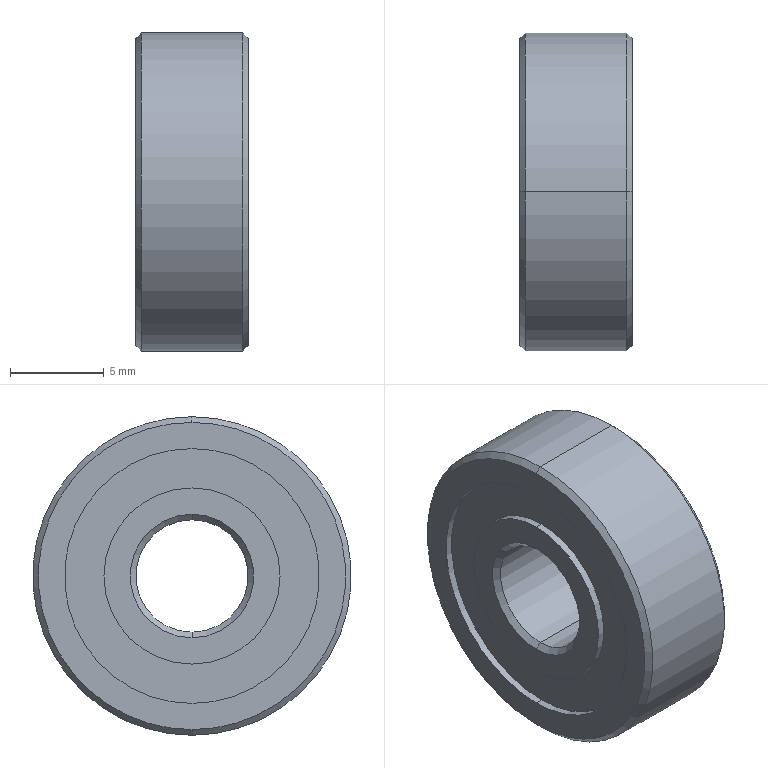Part | SolidWorks | features BaseBody 1 | 1 solid | 26 faces | box 6 x 17 x 17 mm | volume 1125 mm3 | cylinder 12 | cone 8 | plane 6 | commonest cylinder face diameters 9.4 x4 13.6 x4 6 x2 17 x2
STEP:
#1=CARTESIAN_POINT('',(2.7,0.,8.5));
#2=VERTEX_POINT('',#1);
#3=CARTESIAN_POINT('',(2.7,0.,-8.5));
#4=VERTEX_POINT('',#3);
#5=CARTESIAN_POINT('',(2.7,0.,0.));
#6=DIRECTION('',(-1.,0.,0.));
#7=DIRECTION('',(0.,0.,1.));
#8=AXIS2_PLACEMENT_3D('',#5,#6,#7);
#9=CIRCLE('',#8,8.5);
#10=EDGE_CURVE('',#2,#4,#9,.T.);
#11=ORIENTED_EDGE('',*,*,#10,.T.);
#12=CARTESIAN_POINT('',(-2.7,0.,-8.5));
#13=VERTEX_POINT('',#12);
#14=CARTESIAN_POINT('',(3.,0.,-8.5));
#15=DIRECTION('',(-1.,0.,0.));
#16=VECTOR('',#15,1000.);
#17=LINE('',#14,#16);
#18=EDGE_CURVE('',#4,#13,#17,.T.);
#19=ORIENTED_EDGE('',*,*,#18,.T.);
#20=CARTESIAN_POINT('',(-2.7,0.,8.5));
#21=VERTEX_POINT('',#20);
#22=CARTESIAN_POINT('',(-2.7,0.,0.));
#23=DIRECTION('',(1.,0.,0.));
#24=DIRECTION('',(0.,0.,1.));
#25=AXIS2_PLACEMENT_3D('',#22,#23,#24);
#26=CIRCLE('',#25,8.5);
#27=EDGE_CURVE('',#13,#21,#26,.T.);
#28=ORIENTED_EDGE('',*,*,#27,.T.);
#29=CARTESIAN_POINT('',(3.,0.,8.5));
#30=DIRECTION('',(-1.,0.,0.));
#31=VECTOR('',#30,1000.);
#32=LINE('',#29,#31);
#33=EDGE_CURVE('',#2,#21,#32,.T.);
#34=ORIENTED_EDGE('',*,*,#33,.F.);
#35=EDGE_LOOP('',(#11,#19,#28,#34));
#36=FACE_OUTER_BOUND('',#35,.T.);
#37=CARTESIAN_POINT('',(3.,0.,0.));
#38=DIRECTION('',(-1.,0.,0.));
#39=DIRECTION('',(0.,0.,1.));
#40=AXIS2_PLACEMENT_3D('',#37,#38,#39);
#41=CYLINDRICAL_SURFACE('',#40,8.5);
#42=ADVANCED_FACE('',(#36),#41,.T.);
#43=CARTESIAN_POINT('',(3.,0.,8.2));
#44=VERTEX_POINT('',#43);
#45=CARTESIAN_POINT('',(3.,0.,-8.2));
#46=VERTEX_POINT('',#45);
#47=CARTESIAN_POINT('',(3.,0.,0.));
#48=DIRECTION('',(-1.,0.,0.));
#49=DIRECTION('',(0.,0.,1.));
#50=AXIS2_PLACEMENT_3D('',#47,#48,#49);
#51=CIRCLE('',#50,8.2);
#52=EDGE_CURVE('',#44,#46,#51,.T.);
#53=ORIENTED_EDGE('',*,*,#52,.T.);
#54=CARTESIAN_POINT('',(2.7,0.,-8.5));
#55=DIRECTION('',(-0.7071,0.,-0.7071));
#56=VECTOR('',#55,1000.);
#57=LINE('',#54,#56);
#58=EDGE_CURVE('',#46,#4,#57,.T.);
#59=ORIENTED_EDGE('',*,*,#58,.T.);
#60=ORIENTED_EDGE('',*,*,#10,.F.);
#61=CARTESIAN_POINT('',(2.7,0.,8.5));
#62=DIRECTION('',(-0.7071,0.,0.7071));
#63=VECTOR('',#62,1000.);
#64=LINE('',#61,#63);
#65=EDGE_CURVE('',#44,#2,#64,.T.);
#66=ORIENTED_EDGE('',*,*,#65,.F.);
#67=EDGE_LOOP('',(#53,#59,#60,#66));
#68=FACE_OUTER_BOUND('',#67,.T.);
#69=CARTESIAN_POINT('',(2.7,0.,0.));
#70=DIRECTION('',(-1.,0.,0.));
#71=DIRECTION('',(0.,0.,1.));
#72=AXIS2_PLACEMENT_3D('',#69,#70,#71);
#73=CONICAL_SURFACE('',#72,8.5,0.7854);
#74=ADVANCED_FACE('',(#68),#73,.T.);
#75=CARTESIAN_POINT('',(-3.,0.,-8.2));
#76=VERTEX_POINT('',#75);
#77=CARTESIAN_POINT('',(-3.,0.,8.2));
#78=VERTEX_POINT('',#77);
#79=CARTESIAN_POINT('',(-3.,0.,0.));
#80=DIRECTION('',(1.,0.,0.));
#81=DIRECTION('',(0.,0.,-1.));
#82=AXIS2_PLACEMENT_3D('',#79,#80,#81);
#83=CIRCLE('',#82,8.2);
#84=EDGE_CURVE('',#76,#78,#83,.T.);
#85=ORIENTED_EDGE('',*,*,#84,.T.);
#86=CARTESIAN_POINT('',(-2.7,0.,8.5));
#87=DIRECTION('',(0.7071,0.,0.7071));
#88=VECTOR('',#87,1000.);
#89=LINE('',#86,#88);
#90=EDGE_CURVE('',#78,#21,#89,.T.);
#91=ORIENTED_EDGE('',*,*,#90,.T.);
#92=ORIENTED_EDGE('',*,*,#27,.F.);
#93=CARTESIAN_POINT('',(-2.7,0.,-8.5));
#94=DIRECTION('',(0.7071,0.,-0.7071));
#95=VECTOR('',#94,1000.);
#96=LINE('',#93,#95);
#97=EDGE_CURVE('',#76,#13,#96,.T.);
#98=ORIENTED_EDGE('',*,*,#97,.F.);
#99=EDGE_LOOP('',(#85,#91,#92,#98));
#100=FACE_OUTER_BOUND('',#99,.T.);
#101=CARTESIAN_POINT('',(-2.7,0.,0.));
#102=DIRECTION('',(1.,0.,0.));
#103=DIRECTION('',(0.,0.,-1.));
#104=AXIS2_PLACEMENT_3D('',#101,#102,#103);
#105=CONICAL_SURFACE('',#104,8.5,0.7854);
#106=ADVANCED_FACE('',(#100),#105,.T.);
#107=CARTESIAN_POINT('',(3.,0.,-6.8));
#108=VERTEX_POINT('',#107);
#109=CARTESIAN_POINT('',(3.,0.,6.8));
#110=VERTEX_POINT('',#109);
#111=CARTESIAN_POINT('',(3.,0.,0.));
#112=DIRECTION('',(-1.,0.,0.));
#113=DIRECTION('',(0.,0.,1.));
#114=AXIS2_PLACEMENT_3D('',#111,#112,#113);
#115=CIRCLE('',#114,6.8);
#116=EDGE_CURVE('',#108,#110,#115,.T.);
#117=ORIENTED_EDGE('',*,*,#116,.F.);
#118=CARTESIAN_POINT('',(2.6,0.,-6.8));
#119=VERTEX_POINT('',#118);
#120=CARTESIAN_POINT('',(3.,0.,-6.8));
#121=DIRECTION('',(-1.,0.,0.));
#122=VECTOR('',#121,1000.);
#123=LINE('',#120,#122);
#124=EDGE_CURVE('',#108,#119,#123,.T.);
#125=ORIENTED_EDGE('',*,*,#124,.T.);
#126=CARTESIAN_POINT('',(2.6,0.,6.8));
#127=VERTEX_POINT('',#126);
#128=CARTESIAN_POINT('',(2.6,0.,0.));
#129=DIRECTION('',(1.,0.,0.));
#130=DIRECTION('',(0.,0.,1.));
#131=AXIS2_PLACEMENT_3D('',#128,#129,#130);
#132=CIRCLE('',#131,6.8);
#133=EDGE_CURVE('',#127,#119,#132,.T.);
#134=ORIENTED_EDGE('',*,*,#133,.F.);
#135=CARTESIAN_POINT('',(3.,0.,6.8));
#136=DIRECTION('',(-1.,0.,0.));
#137=VECTOR('',#136,1000.);
#138=LINE('',#135,#137);
#139=EDGE_CURVE('',#110,#127,#138,.T.);
#140=ORIENTED_EDGE('',*,*,#139,.F.);
#141=EDGE_LOOP('',(#117,#125,#134,#140));
#142=FACE_OUTER_BOUND('',#141,.T.);
#143=CARTESIAN_POINT('',(3.,0.,0.));
#144=DIRECTION('',(-1.,0.,0.));
#145=DIRECTION('',(0.,0.,1.));
#146=AXIS2_PLACEMENT_3D('',#143,#144,#145);
#147=CYLINDRICAL_SURFACE('',#146,6.8);
#148=ADVANCED_FACE('',(#142),#147,.F.);
#149=CARTESIAN_POINT('',(-2.6,0.,-6.8));
#150=VERTEX_POINT('',#149);
#151=CARTESIAN_POINT('',(-2.6,0.,6.8));
#152=VERTEX_POINT('',#151);
#153=CARTESIAN_POINT('',(-2.6,0.,0.));
#154=DIRECTION('',(-1.,0.,0.));
#155=DIRECTION('',(0.,0.,1.));
#156=AXIS2_PLACEMENT_3D('',#153,#154,#155);
#157=CIRCLE('',#156,6.8);
#158=EDGE_CURVE('',#150,#152,#157,.T.);
#159=ORIENTED_EDGE('',*,*,#158,.F.);
#160=CARTESIAN_POINT('',(-3.,0.,-6.8));
#161=VERTEX_POINT('',#160);
#162=CARTESIAN_POINT('',(3.,0.,-6.8));
#163=DIRECTION('',(-1.,0.,0.));
#164=VECTOR('',#163,1000.);
#165=LINE('',#162,#164);
#166=EDGE_CURVE('',#150,#161,#165,.T.);
#167=ORIENTED_EDGE('',*,*,#166,.T.);
#168=CARTESIAN_POINT('',(-3.,0.,6.8));
#169=VERTEX_POINT('',#168);
#170=CARTESIAN_POINT('',(-3.,0.,0.));
#171=DIRECTION('',(1.,0.,0.));
#172=DIRECTION('',(0.,0.,1.));
#173=AXIS2_PLACEMENT_3D('',#170,#171,#172);
#174=CIRCLE('',#173,6.8);
#175=EDGE_CURVE('',#169,#161,#174,.T.);
#176=ORIENTED_EDGE('',*,*,#175,.F.);
#177=CARTESIAN_POINT('',(3.,0.,6.8));
#178=DIRECTION('',(-1.,0.,0.));
#179=VECTOR('',#178,1000.);
#180=LINE('',#177,#179);
#181=EDGE_CURVE('',#152,#169,#180,.T.);
#182=ORIENTED_EDGE('',*,*,#181,.F.);
#183=EDGE_LOOP('',(#159,#167,#176,#182));
#184=FACE_OUTER_BOUND('',#183,.T.);
#185=CARTESIAN_POINT('',(3.,0.,0.));
#186=DIRECTION('',(-1.,0.,0.));
#187=DIRECTION('',(0.,0.,1.));
#188=AXIS2_PLACEMENT_3D('',#185,#186,#187);
#189=CYLINDRICAL_SURFACE('',#188,6.8);
#190=ADVANCED_FACE('',(#184),#189,.F.);
#191=CARTESIAN_POINT('',(3.,0.,4.7));
#192=VERTEX_POINT('',#191);
#193=CARTESIAN_POINT('',(3.,0.,-4.7));
#194=VERTEX_POINT('',#193);
#195=CARTESIAN_POINT('',(3.,0.,0.));
#196=DIRECTION('',(-1.,0.,0.));
#197=DIRECTION('',(0.,0.,1.));
#198=AXIS2_PLACEMENT_3D('',#195,#196,#197);
#199=CIRCLE('',#198,4.7);
#200=EDGE_CURVE('',#192,#194,#199,.T.);
#201=ORIENTED_EDGE('',*,*,#200,.T.);
#202=CARTESIAN_POINT('',(2.6,0.,-4.7));
#203=VERTEX_POINT('',#202);
#204=CARTESIAN_POINT('',(3.,0.,-4.7));
#205=DIRECTION('',(-1.,0.,0.));
#206=VECTOR('',#205,1000.);
#207=LINE('',#204,#206);
#208=EDGE_CURVE('',#194,#203,#207,.T.);
#209=ORIENTED_EDGE('',*,*,#208,.T.);
#210=CARTESIAN_POINT('',(2.6,0.,4.7));
#211=VERTEX_POINT('',#210);
#212=CARTESIAN_POINT('',(2.6,0.,0.));
#213=DIRECTION('',(-1.,0.,0.));
#214=DIRECTION('',(0.,0.,1.));
#215=AXIS2_PLACEMENT_3D('',#212,#213,#214);
#216=CIRCLE('',#215,4.7);
#217=EDGE_CURVE('',#211,#203,#216,.T.);
#218=ORIENTED_EDGE('',*,*,#217,.F.);
#219=CARTESIAN_POINT('',(3.,0.,4.7));
#220=DIRECTION('',(-1.,0.,0.));
#221=VECTOR('',#220,1000.);
#222=LINE('',#219,#221);
#223=EDGE_CURVE('',#192,#211,#222,.T.);
#224=ORIENTED_EDGE('',*,*,#223,.F.);
#225=EDGE_LOOP('',(#201,#209,#218,#224));
#226=FACE_OUTER_BOUND('',#225,.T.);
#227=CARTESIAN_POINT('',(3.,0.,0.));
#228=DIRECTION('',(-1.,0.,0.));
#229=DIRECTION('',(0.,0.,1.));
#230=AXIS2_PLACEMENT_3D('',#227,#228,#229);
#231=CYLINDRICAL_SURFACE('',#230,4.7);
#232=ADVANCED_FACE('',(#226),#231,.T.);
#233=CARTESIAN_POINT('',(-2.6,0.,-4.7));
#234=VERTEX_POINT('',#233);
#235=CARTESIAN_POINT('',(-2.6,0.,4.7));
#236=VERTEX_POINT('',#235);
#237=CARTESIAN_POINT('',(-2.6,0.,0.));
#238=DIRECTION('',(1.,0.,0.));
#239=DIRECTION('',(0.,0.,1.));
#240=AXIS2_PLACEMENT_3D('',#237,#238,#239);
#241=CIRCLE('',#240,4.7);
#242=EDGE_CURVE('',#234,#236,#241,.T.);
#243=ORIENTED_EDGE('',*,*,#242,.F.);
#244=CARTESIAN_POINT('',(-3.,0.,-4.7));
#245=VERTEX_POINT('',#244);
#246=CARTESIAN_POINT('',(3.,0.,-4.7));
#247=DIRECTION('',(-1.,0.,0.));
#248=VECTOR('',#247,1000.);
#249=LINE('',#246,#248);
#250=EDGE_CURVE('',#234,#245,#249,.T.);
#251=ORIENTED_EDGE('',*,*,#250,.T.);
#252=CARTESIAN_POINT('',(-3.,0.,4.7));
#253=VERTEX_POINT('',#252);
#254=CARTESIAN_POINT('',(-3.,0.,0.));
#255=DIRECTION('',(1.,0.,0.));
#256=DIRECTION('',(0.,0.,1.));
#257=AXIS2_PLACEMENT_3D('',#254,#255,#256);
#258=CIRCLE('',#257,4.7);
#259=EDGE_CURVE('',#245,#253,#258,.T.);
#260=ORIENTED_EDGE('',*,*,#259,.T.);
#261=CARTESIAN_POINT('',(3.,0.,4.7));
#262=DIRECTION('',(-1.,0.,0.));
#263=VECTOR('',#262,1000.);
#264=LINE('',#261,#263);
#265=EDGE_CURVE('',#236,#253,#264,.T.);
#266=ORIENTED_EDGE('',*,*,#265,.F.);
#267=EDGE_LOOP('',(#243,#251,#260,#266));
#268=FACE_OUTER_BOUND('',#267,.T.);
#269=CARTESIAN_POINT('',(3.,0.,0.));
#270=DIRECTION('',(-1.,0.,0.));
#271=DIRECTION('',(0.,0.,1.));
#272=AXIS2_PLACEMENT_3D('',#269,#270,#271);
#273=CYLINDRICAL_SURFACE('',#272,4.7);
#274=ADVANCED_FACE('',(#268),#273,.T.);
#275=CARTESIAN_POINT('',(2.7,0.,3.));
#276=VERTEX_POINT('',#275);
#277=CARTESIAN_POINT('',(2.7,0.,-3.));
#278=VERTEX_POINT('',#277);
#279=CARTESIAN_POINT('',(2.7,0.,0.));
#280=DIRECTION('',(1.,0.,0.));
#281=DIRECTION('',(0.,0.,-1.));
#282=AXIS2_PLACEMENT_3D('',#279,#280,#281);
#283=CIRCLE('',#282,3.);
#284=EDGE_CURVE('',#276,#278,#283,.T.);
#285=ORIENTED_EDGE('',*,*,#284,.F.);
#286=CARTESIAN_POINT('',(3.,0.,3.3));
#287=VERTEX_POINT('',#286);
#288=CARTESIAN_POINT('',(3.,0.,3.3));
#289=DIRECTION('',(0.7071,0.,0.7071));
#290=VECTOR('',#289,1000.);
#291=LINE('',#288,#290);
#292=EDGE_CURVE('',#276,#287,#291,.T.);
#293=ORIENTED_EDGE('',*,*,#292,.T.);
#294=CARTESIAN_POINT('',(3.,0.,-3.3));
#295=VERTEX_POINT('',#294);
#296=CARTESIAN_POINT('',(3.,0.,0.));
#297=DIRECTION('',(-1.,0.,0.));
#298=DIRECTION('',(0.,0.,-1.));
#299=AXIS2_PLACEMENT_3D('',#296,#297,#298);
#300=CIRCLE('',#299,3.3);
#301=EDGE_CURVE('',#295,#287,#300,.T.);
#302=ORIENTED_EDGE('',*,*,#301,.F.);
#303=CARTESIAN_POINT('',(3.,0.,-3.3));
#304=DIRECTION('',(0.7071,0.,-0.7071));
#305=VECTOR('',#304,1000.);
#306=LINE('',#303,#305);
#307=EDGE_CURVE('',#278,#295,#306,.T.);
#308=ORIENTED_EDGE('',*,*,#307,.F.);
#309=EDGE_LOOP('',(#285,#293,#302,#308));
#310=FACE_OUTER_BOUND('',#309,.T.);
#311=CARTESIAN_POINT('',(3.,0.,0.));
#312=DIRECTION('',(1.,0.,0.));
#313=DIRECTION('',(0.,0.,-1.));
#314=AXIS2_PLACEMENT_3D('',#311,#312,#313);
#315=CONICAL_SURFACE('',#314,3.3,0.7854);
#316=ADVANCED_FACE('',(#310),#315,.F.);
#317=CARTESIAN_POINT('',(-2.7,0.,-3.));
#318=VERTEX_POINT('',#317);
#319=CARTESIAN_POINT('',(-2.7,0.,3.));
#320=VERTEX_POINT('',#319);
#321=CARTESIAN_POINT('',(-2.7,0.,0.));
#322=DIRECTION('',(-1.,0.,0.));
#323=DIRECTION('',(0.,0.,1.));
#324=AXIS2_PLACEMENT_3D('',#321,#322,#323);
#325=CIRCLE('',#324,3.);
#326=EDGE_CURVE('',#318,#320,#325,.T.);
#327=ORIENTED_EDGE('',*,*,#326,.F.);
#328=CARTESIAN_POINT('',(-3.,0.,-3.3));
#329=VERTEX_POINT('',#328);
#330=CARTESIAN_POINT('',(-3.,0.,-3.3));
#331=DIRECTION('',(-0.7071,0.,-0.7071));
#332=VECTOR('',#331,1000.);
#333=LINE('',#330,#332);
#334=EDGE_CURVE('',#318,#329,#333,.T.);
#335=ORIENTED_EDGE('',*,*,#334,.T.);
#336=CARTESIAN_POINT('',(-3.,0.,3.3));
#337=VERTEX_POINT('',#336);
#338=CARTESIAN_POINT('',(-3.,0.,0.));
#339=DIRECTION('',(1.,0.,0.));
#340=DIRECTION('',(0.,0.,1.));
#341=AXIS2_PLACEMENT_3D('',#338,#339,#340);
#342=CIRCLE('',#341,3.3);
#343=EDGE_CURVE('',#337,#329,#342,.T.);
#344=ORIENTED_EDGE('',*,*,#343,.F.);
#345=CARTESIAN_POINT('',(-3.,0.,3.3));
#346=DIRECTION('',(-0.7071,0.,0.7071));
#347=VECTOR('',#346,1000.);
#348=LINE('',#345,#347);
#349=EDGE_CURVE('',#320,#337,#348,.T.);
#350=ORIENTED_EDGE('',*,*,#349,.F.);
#351=EDGE_LOOP('',(#327,#335,#344,#350));
#352=FACE_OUTER_BOUND('',#351,.T.);
#353=CARTESIAN_POINT('',(-3.,0.,0.));
#354=DIRECTION('',(-1.,0.,0.));
#355=DIRECTION('',(0.,0.,1.));
#356=AXIS2_PLACEMENT_3D('',#353,#354,#355);
#357=CONICAL_SURFACE('',#356,3.3,0.7854);
#358=ADVANCED_FACE('',(#352),#357,.F.);
#359=ORIENTED_EDGE('',*,*,#284,.T.);
#360=CARTESIAN_POINT('',(3.,0.,-3.));
#361=DIRECTION('',(-1.,0.,0.));
#362=VECTOR('',#361,1000.);
#363=LINE('',#360,#362);
#364=EDGE_CURVE('',#278,#318,#363,.T.);
#365=ORIENTED_EDGE('',*,*,#364,.T.);
#366=ORIENTED_EDGE('',*,*,#326,.T.);
#367=CARTESIAN_POINT('',(3.,0.,3.));
#368=DIRECTION('',(-1.,0.,0.));
#369=VECTOR('',#368,1000.);
#370=LINE('',#367,#369);
#371=EDGE_CURVE('',#276,#320,#370,.T.);
#372=ORIENTED_EDGE('',*,*,#371,.F.);
#373=EDGE_LOOP('',(#359,#365,#366,#372));
#374=FACE_OUTER_BOUND('',#373,.T.);
#375=CARTESIAN_POINT('',(3.,0.,0.));
#376=DIRECTION('',(-1.,0.,0.));
#377=DIRECTION('',(0.,0.,1.));
#378=AXIS2_PLACEMENT_3D('',#375,#376,#377);
#379=CYLINDRICAL_SURFACE('',#378,3.);
#380=ADVANCED_FACE('',(#374),#379,.F.);
#381=ORIENTED_EDGE('',*,*,#18,.F.);
#382=CARTESIAN_POINT('',(2.7,0.,0.));
#383=DIRECTION('',(-1.,0.,0.));
#384=DIRECTION('',(0.,0.,1.));
#385=AXIS2_PLACEMENT_3D('',#382,#383,#384);
#386=CIRCLE('',#385,8.5);
#387=EDGE_CURVE('',#4,#2,#386,.T.);
#388=ORIENTED_EDGE('',*,*,#387,.T.);
#389=ORIENTED_EDGE('',*,*,#33,.T.);
#390=CARTESIAN_POINT('',(-2.7,0.,0.));
#391=DIRECTION('',(1.,0.,0.));
#392=DIRECTION('',(0.,0.,1.));
#393=AXIS2_PLACEMENT_3D('',#390,#391,#392);
#394=CIRCLE('',#393,8.5);
#395=EDGE_CURVE('',#21,#13,#394,.T.);
#396=ORIENTED_EDGE('',*,*,#395,.T.);
#397=EDGE_LOOP('',(#381,#388,#389,#396));
#398=FACE_OUTER_BOUND('',#397,.T.);
#399=CARTESIAN_POINT('',(3.,0.,0.));
#400=DIRECTION('',(-1.,0.,0.));
#401=DIRECTION('',(0.,0.,1.));
#402=AXIS2_PLACEMENT_3D('',#399,#400,#401);
#403=CYLINDRICAL_SURFACE('',#402,8.5);
#404=ADVANCED_FACE('',(#398),#403,.T.);
#405=ORIENTED_EDGE('',*,*,#58,.F.);
#406=CARTESIAN_POINT('',(3.,0.,0.));
#407=DIRECTION('',(-1.,0.,0.));
#408=DIRECTION('',(0.,0.,1.));
#409=AXIS2_PLACEMENT_3D('',#406,#407,#408);
#410=CIRCLE('',#409,8.2);
#411=EDGE_CURVE('',#46,#44,#410,.T.);
#412=ORIENTED_EDGE('',*,*,#411,.T.);
#413=ORIENTED_EDGE('',*,*,#65,.T.);
#414=ORIENTED_EDGE('',*,*,#387,.F.);
#415=EDGE_LOOP('',(#405,#412,#413,#414));
#416=FACE_OUTER_BOUND('',#415,.T.);
#417=CARTESIAN_POINT('',(2.7,0.,0.));
#418=DIRECTION('',(-1.,0.,0.));
#419=DIRECTION('',(0.,0.,1.));
#420=AXIS2_PLACEMENT_3D('',#417,#418,#419);
#421=CONICAL_SURFACE('',#420,8.5,0.7854);
#422=ADVANCED_FACE('',(#416),#421,.T.);
#423=ORIENTED_EDGE('',*,*,#90,.F.);
#424=CARTESIAN_POINT('',(-3.,0.,0.));
#425=DIRECTION('',(1.,0.,0.));
#426=DIRECTION('',(0.,0.,-1.));
#427=AXIS2_PLACEMENT_3D('',#424,#425,#426);
#428=CIRCLE('',#427,8.2);
#429=EDGE_CURVE('',#78,#76,#428,.T.);
#430=ORIENTED_EDGE('',*,*,#429,.T.);
#431=ORIENTED_EDGE('',*,*,#97,.T.);
#432=ORIENTED_EDGE('',*,*,#395,.F.);
#433=EDGE_LOOP('',(#423,#430,#431,#432));
#434=FACE_OUTER_BOUND('',#433,.T.);
#435=CARTESIAN_POINT('',(-2.7,0.,0.));
#436=DIRECTION('',(1.,0.,0.));
#437=DIRECTION('',(0.,0.,-1.));
#438=AXIS2_PLACEMENT_3D('',#435,#436,#437);
#439=CONICAL_SURFACE('',#438,8.5,0.7854);
#440=ADVANCED_FACE('',(#434),#439,.T.);
#441=CARTESIAN_POINT('',(3.,0.,0.));
#442=DIRECTION('',(-1.,0.,0.));
#443=DIRECTION('',(0.,0.,1.));
#444=AXIS2_PLACEMENT_3D('',#441,#442,#443);
#445=CIRCLE('',#444,6.8);
#446=EDGE_CURVE('',#110,#108,#445,.T.);
#447=ORIENTED_EDGE('',*,*,#446,.T.);
#448=ORIENTED_EDGE('',*,*,#116,.T.);
#449=EDGE_LOOP('',(#447,#448));
#450=FACE_BOUND('',#449,.T.);
#451=ORIENTED_EDGE('',*,*,#52,.F.);
#452=ORIENTED_EDGE('',*,*,#411,.F.);
#453=EDGE_LOOP('',(#451,#452));
#454=FACE_OUTER_BOUND('',#453,.T.);
#455=CARTESIAN_POINT('',(3.,6.8,0.));
#456=DIRECTION('',(1.,0.,0.));
#457=DIRECTION('',(0.,0.,-1.));
#458=AXIS2_PLACEMENT_3D('',#455,#456,#457);
#459=PLANE('',#458);
#460=ADVANCED_FACE('',(#450,#454),#459,.T.);
#461=ORIENTED_EDGE('',*,*,#84,.F.);
#462=ORIENTED_EDGE('',*,*,#429,.F.);
#463=EDGE_LOOP('',(#461,#462));
#464=FACE_OUTER_BOUND('',#463,.T.);
#465=ORIENTED_EDGE('',*,*,#175,.T.);
#466=CARTESIAN_POINT('',(-3.,0.,0.));
#467=DIRECTION('',(1.,0.,0.));
#468=DIRECTION('',(0.,0.,1.));
#469=AXIS2_PLACEMENT_3D('',#466,#467,#468);
#470=CIRCLE('',#469,6.8);
#471=EDGE_CURVE('',#161,#169,#470,.T.);
#472=ORIENTED_EDGE('',*,*,#471,.T.);
#473=EDGE_LOOP('',(#465,#472));
#474=FACE_BOUND('',#473,.T.);
#475=CARTESIAN_POINT('',(-3.,8.2,0.));
#476=DIRECTION('',(-1.,0.,0.));
#477=DIRECTION('',(0.,0.,1.));
#478=AXIS2_PLACEMENT_3D('',#475,#476,#477);
#479=PLANE('',#478);
#480=ADVANCED_FACE('',(#464,#474),#479,.T.);
#481=ORIENTED_EDGE('',*,*,#124,.F.);
#482=ORIENTED_EDGE('',*,*,#446,.F.);
#483=ORIENTED_EDGE('',*,*,#139,.T.);
#484=CARTESIAN_POINT('',(2.6,0.,0.));
#485=DIRECTION('',(1.,0.,0.));
#486=DIRECTION('',(0.,0.,1.));
#487=AXIS2_PLACEMENT_3D('',#484,#485,#486);
#488=CIRCLE('',#487,6.8);
#489=EDGE_CURVE('',#119,#127,#488,.T.);
#490=ORIENTED_EDGE('',*,*,#489,.F.);
#491=EDGE_LOOP('',(#481,#482,#483,#490));
#492=FACE_OUTER_BOUND('',#491,.T.);
#493=CARTESIAN_POINT('',(3.,0.,0.));
#494=DIRECTION('',(-1.,0.,0.));
#495=DIRECTION('',(0.,0.,1.));
#496=AXIS2_PLACEMENT_3D('',#493,#494,#495);
#497=CYLINDRICAL_SURFACE('',#496,6.8);
#498=ADVANCED_FACE('',(#492),#497,.F.);
#499=ORIENTED_EDGE('',*,*,#166,.F.);
#500=CARTESIAN_POINT('',(-2.6,0.,0.));
#501=DIRECTION('',(-1.,0.,0.));
#502=DIRECTION('',(0.,0.,1.));
#503=AXIS2_PLACEMENT_3D('',#500,#501,#502);
#504=CIRCLE('',#503,6.8);
#505=EDGE_CURVE('',#152,#150,#504,.T.);
#506=ORIENTED_EDGE('',*,*,#505,.F.);
#507=ORIENTED_EDGE('',*,*,#181,.T.);
#508=ORIENTED_EDGE('',*,*,#471,.F.);
#509=EDGE_LOOP('',(#499,#506,#507,#508));
#510=FACE_OUTER_BOUND('',#509,.T.);
#511=CARTESIAN_POINT('',(3.,0.,0.));
#512=DIRECTION('',(-1.,0.,0.));
#513=DIRECTION('',(0.,0.,1.));
#514=AXIS2_PLACEMENT_3D('',#511,#512,#513);
#515=CYLINDRICAL_SURFACE('',#514,6.8);
#516=ADVANCED_FACE('',(#510),#515,.F.);
#517=ORIENTED_EDGE('',*,*,#217,.T.);
#518=CARTESIAN_POINT('',(2.6,0.,0.));
#519=DIRECTION('',(-1.,0.,0.));
#520=DIRECTION('',(0.,0.,1.));
#521=AXIS2_PLACEMENT_3D('',#518,#519,#520);
#522=CIRCLE('',#521,4.7);
#523=EDGE_CURVE('',#203,#211,#522,.T.);
#524=ORIENTED_EDGE('',*,*,#523,.T.);
#525=EDGE_LOOP('',(#517,#524));
#526=FACE_BOUND('',#525,.T.);
#527=ORIENTED_EDGE('',*,*,#133,.T.);
#528=ORIENTED_EDGE('',*,*,#489,.T.);
#529=EDGE_LOOP('',(#527,#528));
#530=FACE_OUTER_BOUND('',#529,.T.);
#531=CARTESIAN_POINT('',(2.6,4.7,0.));
#532=DIRECTION('',(1.,0.,0.));
#533=DIRECTION('',(0.,0.,-1.));
#534=AXIS2_PLACEMENT_3D('',#531,#532,#533);
#535=PLANE('',#534);
#536=ADVANCED_FACE('',(#526,#530),#535,.T.);
#537=ORIENTED_EDGE('',*,*,#505,.T.);
#538=ORIENTED_EDGE('',*,*,#158,.T.);
#539=EDGE_LOOP('',(#537,#538));
#540=FACE_OUTER_BOUND('',#539,.T.);
#541=CARTESIAN_POINT('',(-2.6,0.,0.));
#542=DIRECTION('',(1.,0.,0.));
#543=DIRECTION('',(0.,0.,1.));
#544=AXIS2_PLACEMENT_3D('',#541,#542,#543);
#545=CIRCLE('',#544,4.7);
#546=EDGE_CURVE('',#236,#234,#545,.T.);
#547=ORIENTED_EDGE('',*,*,#546,.T.);
#548=ORIENTED_EDGE('',*,*,#242,.T.);
#549=EDGE_LOOP('',(#547,#548));
#550=FACE_BOUND('',#549,.T.);
#551=CARTESIAN_POINT('',(-2.6,6.8,0.));
#552=DIRECTION('',(-1.,0.,0.));
#553=DIRECTION('',(0.,0.,1.));
#554=AXIS2_PLACEMENT_3D('',#551,#552,#553);
#555=PLANE('',#554);
#556=ADVANCED_FACE('',(#540,#550),#555,.T.);
#557=ORIENTED_EDGE('',*,*,#208,.F.);
#558=CARTESIAN_POINT('',(3.,0.,0.));
#559=DIRECTION('',(-1.,0.,0.));
#560=DIRECTION('',(0.,0.,1.));
#561=AXIS2_PLACEMENT_3D('',#558,#559,#560);
#562=CIRCLE('',#561,4.7);
#563=EDGE_CURVE('',#194,#192,#562,.T.);
#564=ORIENTED_EDGE('',*,*,#563,.T.);
#565=ORIENTED_EDGE('',*,*,#223,.T.);
#566=ORIENTED_EDGE('',*,*,#523,.F.);
#567=EDGE_LOOP('',(#557,#564,#565,#566));
#568=FACE_OUTER_BOUND('',#567,.T.);
#569=CARTESIAN_POINT('',(3.,0.,0.));
#570=DIRECTION('',(-1.,0.,0.));
#571=DIRECTION('',(0.,0.,1.));
#572=AXIS2_PLACEMENT_3D('',#569,#570,#571);
#573=CYLINDRICAL_SURFACE('',#572,4.7);
#574=ADVANCED_FACE('',(#568),#573,.T.);
#575=ORIENTED_EDGE('',*,*,#250,.F.);
#576=ORIENTED_EDGE('',*,*,#546,.F.);
#577=ORIENTED_EDGE('',*,*,#265,.T.);
#578=CARTESIAN_POINT('',(-3.,0.,0.));
#579=DIRECTION('',(1.,0.,0.));
#580=DIRECTION('',(0.,0.,1.));
#581=AXIS2_PLACEMENT_3D('',#578,#579,#580);
#582=CIRCLE('',#581,4.7);
#583=EDGE_CURVE('',#253,#245,#582,.T.);
#584=ORIENTED_EDGE('',*,*,#583,.T.);
#585=EDGE_LOOP('',(#575,#576,#577,#584));
#586=FACE_OUTER_BOUND('',#585,.T.);
#587=CARTESIAN_POINT('',(3.,0.,0.));
#588=DIRECTION('',(-1.,0.,0.));
#589=DIRECTION('',(0.,0.,1.));
#590=AXIS2_PLACEMENT_3D('',#587,#588,#589);
#591=CYLINDRICAL_SURFACE('',#590,4.7);
#592=ADVANCED_FACE('',(#586),#591,.T.);
#593=ORIENTED_EDGE('',*,*,#301,.T.);
#594=CARTESIAN_POINT('',(3.,0.,0.));
#595=DIRECTION('',(-1.,0.,0.));
#596=DIRECTION('',(0.,0.,-1.));
#597=AXIS2_PLACEMENT_3D('',#594,#595,#596);
#598=CIRCLE('',#597,3.3);
#599=EDGE_CURVE('',#287,#295,#598,.T.);
#600=ORIENTED_EDGE('',*,*,#599,.T.);
#601=EDGE_LOOP('',(#593,#600));
#602=FACE_BOUND('',#601,.T.);
#603=ORIENTED_EDGE('',*,*,#200,.F.);
#604=ORIENTED_EDGE('',*,*,#563,.F.);
#605=EDGE_LOOP('',(#603,#604));
#606=FACE_OUTER_BOUND('',#605,.T.);
#607=CARTESIAN_POINT('',(3.,3.3,0.));
#608=DIRECTION('',(1.,0.,0.));
#609=DIRECTION('',(0.,0.,-1.));
#610=AXIS2_PLACEMENT_3D('',#607,#608,#609);
#611=PLANE('',#610);
#612=ADVANCED_FACE('',(#602,#606),#611,.T.);
#613=ORIENTED_EDGE('',*,*,#583,.F.);
#614=ORIENTED_EDGE('',*,*,#259,.F.);
#615=EDGE_LOOP('',(#613,#614));
#616=FACE_OUTER_BOUND('',#615,.T.);
#617=ORIENTED_EDGE('',*,*,#343,.T.);
#618=CARTESIAN_POINT('',(-3.,0.,0.));
#619=DIRECTION('',(1.,0.,0.));
#620=DIRECTION('',(0.,0.,1.));
#621=AXIS2_PLACEMENT_3D('',#618,#619,#620);
#622=CIRCLE('',#621,3.3);
#623=EDGE_CURVE('',#329,#337,#622,.T.);
#624=ORIENTED_EDGE('',*,*,#623,.T.);
#625=EDGE_LOOP('',(#617,#624));
#626=FACE_BOUND('',#625,.T.);
#627=CARTESIAN_POINT('',(-3.,4.7,0.));
#628=DIRECTION('',(-1.,0.,0.));
#629=DIRECTION('',(0.,0.,1.));
#630=AXIS2_PLACEMENT_3D('',#627,#628,#629);
#631=PLANE('',#630);
#632=ADVANCED_FACE('',(#616,#626),#631,.T.);
#633=ORIENTED_EDGE('',*,*,#292,.F.);
#634=CARTESIAN_POINT('',(2.7,0.,0.));
#635=DIRECTION('',(1.,0.,0.));
#636=DIRECTION('',(0.,0.,-1.));
#637=AXIS2_PLACEMENT_3D('',#634,#635,#636);
#638=CIRCLE('',#637,3.);
#639=EDGE_CURVE('',#278,#276,#638,.T.);
#640=ORIENTED_EDGE('',*,*,#639,.F.);
#641=ORIENTED_EDGE('',*,*,#307,.T.);
#642=ORIENTED_EDGE('',*,*,#599,.F.);
#643=EDGE_LOOP('',(#633,#640,#641,#642));
#644=FACE_OUTER_BOUND('',#643,.T.);
#645=CARTESIAN_POINT('',(3.,0.,0.));
#646=DIRECTION('',(1.,0.,0.));
#647=DIRECTION('',(0.,0.,-1.));
#648=AXIS2_PLACEMENT_3D('',#645,#646,#647);
#649=CONICAL_SURFACE('',#648,3.3,0.7854);
#650=ADVANCED_FACE('',(#644),#649,.F.);
#651=ORIENTED_EDGE('',*,*,#334,.F.);
#652=CARTESIAN_POINT('',(-2.7,0.,0.));
#653=DIRECTION('',(-1.,0.,0.));
#654=DIRECTION('',(0.,0.,1.));
#655=AXIS2_PLACEMENT_3D('',#652,#653,#654);
#656=CIRCLE('',#655,3.);
#657=EDGE_CURVE('',#320,#318,#656,.T.);
#658=ORIENTED_EDGE('',*,*,#657,.F.);
#659=ORIENTED_EDGE('',*,*,#349,.T.);
#660=ORIENTED_EDGE('',*,*,#623,.F.);
#661=EDGE_LOOP('',(#651,#658,#659,#660));
#662=FACE_OUTER_BOUND('',#661,.T.);
#663=CARTESIAN_POINT('',(-3.,0.,0.));
#664=DIRECTION('',(-1.,0.,0.));
#665=DIRECTION('',(0.,0.,1.));
#666=AXIS2_PLACEMENT_3D('',#663,#664,#665);
#667=CONICAL_SURFACE('',#666,3.3,0.7854);
#668=ADVANCED_FACE('',(#662),#667,.F.);
#669=ORIENTED_EDGE('',*,*,#364,.F.);
#670=ORIENTED_EDGE('',*,*,#639,.T.);
#671=ORIENTED_EDGE('',*,*,#371,.T.);
#672=ORIENTED_EDGE('',*,*,#657,.T.);
#673=EDGE_LOOP('',(#669,#670,#671,#672));
#674=FACE_OUTER_BOUND('',#673,.T.);
#675=CARTESIAN_POINT('',(3.,0.,0.));
#676=DIRECTION('',(-1.,0.,0.));
#677=DIRECTION('',(0.,0.,1.));
#678=AXIS2_PLACEMENT_3D('',#675,#676,#677);
#679=CYLINDRICAL_SURFACE('',#678,3.);
#680=ADVANCED_FACE('',(#674),#679,.F.);
#681=CLOSED_SHELL('',(#42,#74,#106,#148,#190,#232,#274,#316,#358,#380,#404,#422,#440,#460,#480,#498,#516,#536,#556,#574,#592,#612,#632,#650,#668,#680));
#682=MANIFOLD_SOLID_BREP('',#681);
#683=CARTESIAN_POINT('',(0.,0.,0.));
#684=DIRECTION('',(0.,0.,1.));
#685=DIRECTION('',(1.,0.,0.));
#686=AXIS2_PLACEMENT_3D('',#683,#684,#685);
#687=(LENGTH_UNIT()NAMED_UNIT(*)SI_UNIT(.MILLI.,.METRE.));
#688=UNCERTAINTY_MEASURE_WITH_UNIT(LENGTH_MEASURE(0.00001),#687,'','');
#689=(NAMED_UNIT(*)PLANE_ANGLE_UNIT()SI_UNIT($,.RADIAN.));
#690=(NAMED_UNIT(*)SI_UNIT($,.STERADIAN.)SOLID_ANGLE_UNIT());
#691=(GEOMETRIC_REPRESENTATION_CONTEXT(3)GLOBAL_UNCERTAINTY_ASSIGNED_CONTEXT((#688))GLOBAL_UNIT_ASSIGNED_CONTEXT((#687,#689,#690))REPRESENTATION_CONTEXT('',''));
#692=ADVANCED_BREP_SHAPE_REPRESENTATION('',(#682,#686),#691);